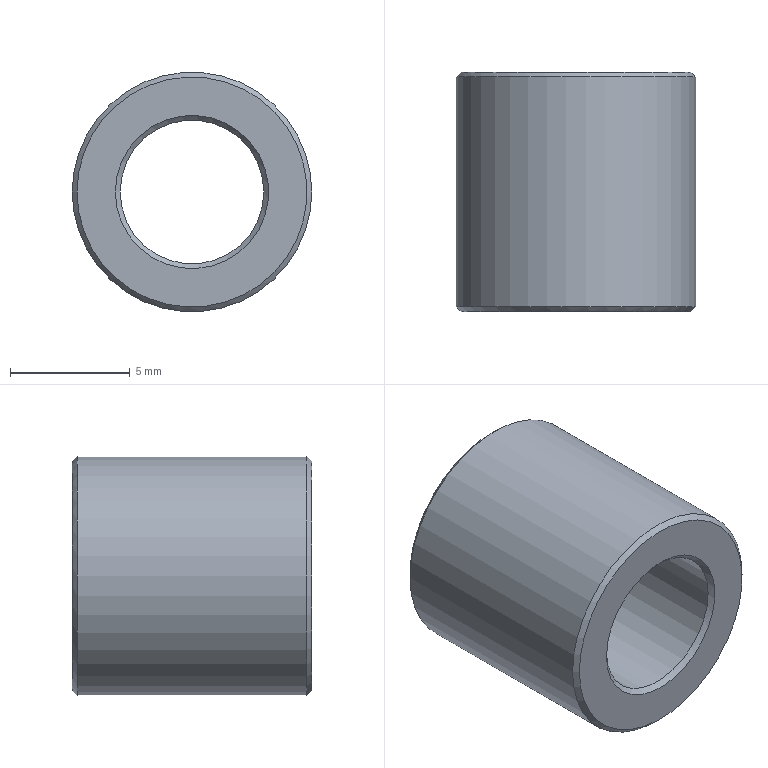Part | NX | features 5003_026_C-KNCLA6-10-10 2 | 1 solid | 8 faces | box 10 x 10 x 10 mm | volume 500.644 mm3 | cone 4 | plane 2 | cylinder 2 | commonest cylinder face diameters 6 x1 10 x1
STEP:
#1=CARTESIAN_POINT('',(-221.575,-608.6,-110.5));
#2=VERTEX_POINT('',#1);
#3=CARTESIAN_POINT('',(-216.775,-608.6,-110.5));
#4=DIRECTION('',(0.,1.,0.));
#5=DIRECTION('',(-1.,0.,0.));
#6=AXIS2_PLACEMENT_3D('',#3,#4,#5);
#7=CIRCLE('',#6,4.8);
#8=EDGE_CURVE('',#2,#2,#7,.F.);
#9=ORIENTED_EDGE('',*,*,#8,.T.);
#10=EDGE_LOOP('',(#9));
#11=FACE_BOUND('',#10,.T.);
#12=CARTESIAN_POINT('',(-219.975,-608.6,-110.5));
#13=VERTEX_POINT('',#12);
#14=CARTESIAN_POINT('',(-216.775,-608.6,-110.5));
#15=DIRECTION('',(0.,1.,0.));
#16=DIRECTION('',(-1.,0.,0.));
#17=AXIS2_PLACEMENT_3D('',#14,#15,#16);
#18=CIRCLE('',#17,3.2);
#19=EDGE_CURVE('',#13,#13,#18,.T.);
#20=ORIENTED_EDGE('',*,*,#19,.T.);
#21=EDGE_LOOP('',(#20));
#22=FACE_BOUND('',#21,.T.);
#23=CARTESIAN_POINT('',(-219.775,-608.6,-110.5));
#24=DIRECTION('',(0.,1.,0.));
#25=DIRECTION('',(-1.,0.,0.));
#26=AXIS2_PLACEMENT_3D('',#23,#24,#25);
#27=PLANE('',#26);
#28=ADVANCED_FACE('',(#11,#22),#27,.F.);
#29=CARTESIAN_POINT('',(-221.775,-608.4,-110.5));
#30=VERTEX_POINT('',#29);
#31=CARTESIAN_POINT('',(-216.775,-608.4,-110.5));
#32=DIRECTION('',(0.,1.,0.));
#33=DIRECTION('',(-1.,0.,0.));
#34=AXIS2_PLACEMENT_3D('',#31,#32,#33);
#35=CIRCLE('',#34,5.);
#36=EDGE_CURVE('',#30,#30,#35,.T.);
#37=ORIENTED_EDGE('',*,*,#36,.T.);
#38=EDGE_LOOP('',(#37));
#39=FACE_BOUND('',#38,.T.);
#40=CARTESIAN_POINT('',(-211.775,-598.8,-110.5));
#41=VERTEX_POINT('',#40);
#42=CARTESIAN_POINT('',(-216.775,-598.8,-110.5));
#43=DIRECTION('',(0.,-1.,0.));
#44=DIRECTION('',(1.,0.,0.));
#45=AXIS2_PLACEMENT_3D('',#42,#43,#44);
#46=CIRCLE('',#45,5.);
#47=EDGE_CURVE('',#41,#41,#46,.T.);
#48=ORIENTED_EDGE('',*,*,#47,.T.);
#49=EDGE_LOOP('',(#48));
#50=FACE_BOUND('',#49,.T.);
#51=CARTESIAN_POINT('',(-216.775,-608.6,-110.5));
#52=DIRECTION('',(0.,-1.,0.));
#53=DIRECTION('',(1.,0.,0.));
#54=AXIS2_PLACEMENT_3D('',#51,#52,#53);
#55=CYLINDRICAL_SURFACE('',#54,5.);
#56=ADVANCED_FACE('',(#39,#50),#55,.T.);
#57=CARTESIAN_POINT('',(-213.575,-598.6,-110.5));
#58=VERTEX_POINT('',#57);
#59=CARTESIAN_POINT('',(-216.775,-598.6,-110.5));
#60=DIRECTION('',(0.,-1.,0.));
#61=DIRECTION('',(1.,0.,0.));
#62=AXIS2_PLACEMENT_3D('',#59,#60,#61);
#63=CIRCLE('',#62,3.2);
#64=EDGE_CURVE('',#58,#58,#63,.T.);
#65=ORIENTED_EDGE('',*,*,#64,.T.);
#66=EDGE_LOOP('',(#65));
#67=FACE_BOUND('',#66,.T.);
#68=CARTESIAN_POINT('',(-211.975,-598.6,-110.5));
#69=VERTEX_POINT('',#68);
#70=CARTESIAN_POINT('',(-216.775,-598.6,-110.5));
#71=DIRECTION('',(0.,-1.,0.));
#72=DIRECTION('',(1.,0.,0.));
#73=AXIS2_PLACEMENT_3D('',#70,#71,#72);
#74=CIRCLE('',#73,4.8);
#75=EDGE_CURVE('',#69,#69,#74,.F.);
#76=ORIENTED_EDGE('',*,*,#75,.T.);
#77=EDGE_LOOP('',(#76));
#78=FACE_BOUND('',#77,.T.);
#79=CARTESIAN_POINT('',(-219.775,-598.6,-110.5));
#80=DIRECTION('',(0.,-1.,0.));
#81=DIRECTION('',(1.,0.,0.));
#82=AXIS2_PLACEMENT_3D('',#79,#80,#81);
#83=PLANE('',#82);
#84=ADVANCED_FACE('',(#67,#78),#83,.F.);
#85=CARTESIAN_POINT('',(-219.775,-608.4,-110.5));
#86=VERTEX_POINT('',#85);
#87=CARTESIAN_POINT('',(-216.775,-608.4,-110.5));
#88=DIRECTION('',(0.,1.,0.));
#89=DIRECTION('',(-1.,0.,0.));
#90=AXIS2_PLACEMENT_3D('',#87,#88,#89);
#91=CIRCLE('',#90,3.);
#92=EDGE_CURVE('',#86,#86,#91,.F.);
#93=ORIENTED_EDGE('',*,*,#92,.T.);
#94=EDGE_LOOP('',(#93));
#95=FACE_BOUND('',#94,.T.);
#96=CARTESIAN_POINT('',(-213.775,-598.8,-110.5));
#97=VERTEX_POINT('',#96);
#98=CARTESIAN_POINT('',(-216.775,-598.8,-110.5));
#99=DIRECTION('',(0.,-1.,0.));
#100=DIRECTION('',(1.,0.,0.));
#101=AXIS2_PLACEMENT_3D('',#98,#99,#100);
#102=CIRCLE('',#101,3.);
#103=EDGE_CURVE('',#97,#97,#102,.F.);
#104=ORIENTED_EDGE('',*,*,#103,.T.);
#105=EDGE_LOOP('',(#104));
#106=FACE_BOUND('',#105,.T.);
#107=CARTESIAN_POINT('',(-216.775,-608.6,-110.5));
#108=DIRECTION('',(0.,-1.,0.));
#109=DIRECTION('',(1.,0.,0.));
#110=AXIS2_PLACEMENT_3D('',#107,#108,#109);
#111=CYLINDRICAL_SURFACE('',#110,3.);
#112=ADVANCED_FACE('',(#95,#106),#111,.F.);
#113=ORIENTED_EDGE('',*,*,#36,.F.);
#114=EDGE_LOOP('',(#113));
#115=FACE_BOUND('',#114,.T.);
#116=ORIENTED_EDGE('',*,*,#8,.F.);
#117=EDGE_LOOP('',(#116));
#118=FACE_BOUND('',#117,.T.);
#119=CARTESIAN_POINT('',(-216.775,-608.6,-110.5));
#120=DIRECTION('',(0.,1.,0.));
#121=DIRECTION('',(-1.,0.,0.));
#122=AXIS2_PLACEMENT_3D('',#119,#120,#121);
#123=CONICAL_SURFACE('',#122,4.8,0.7854);
#124=ADVANCED_FACE('',(#115,#118),#123,.T.);
#125=ORIENTED_EDGE('',*,*,#19,.F.);
#126=EDGE_LOOP('',(#125));
#127=FACE_BOUND('',#126,.T.);
#128=ORIENTED_EDGE('',*,*,#92,.F.);
#129=EDGE_LOOP('',(#128));
#130=FACE_BOUND('',#129,.T.);
#131=CARTESIAN_POINT('',(-216.775,-608.4,-110.5));
#132=DIRECTION('',(0.,-1.,0.));
#133=DIRECTION('',(1.,0.,0.));
#134=AXIS2_PLACEMENT_3D('',#131,#132,#133);
#135=CONICAL_SURFACE('',#134,3.,0.7854);
#136=ADVANCED_FACE('',(#127,#130),#135,.F.);
#137=ORIENTED_EDGE('',*,*,#103,.F.);
#138=EDGE_LOOP('',(#137));
#139=FACE_BOUND('',#138,.T.);
#140=ORIENTED_EDGE('',*,*,#64,.F.);
#141=EDGE_LOOP('',(#140));
#142=FACE_BOUND('',#141,.T.);
#143=CARTESIAN_POINT('',(-216.775,-598.6,-110.5));
#144=DIRECTION('',(0.,1.,0.));
#145=DIRECTION('',(-1.,0.,0.));
#146=AXIS2_PLACEMENT_3D('',#143,#144,#145);
#147=CONICAL_SURFACE('',#146,3.2,0.7854);
#148=ADVANCED_FACE('',(#139,#142),#147,.F.);
#149=ORIENTED_EDGE('',*,*,#75,.F.);
#150=EDGE_LOOP('',(#149));
#151=FACE_BOUND('',#150,.T.);
#152=ORIENTED_EDGE('',*,*,#47,.F.);
#153=EDGE_LOOP('',(#152));
#154=FACE_BOUND('',#153,.T.);
#155=CARTESIAN_POINT('',(-216.775,-598.8,-110.5));
#156=DIRECTION('',(0.,-1.,0.));
#157=DIRECTION('',(1.,0.,0.));
#158=AXIS2_PLACEMENT_3D('',#155,#156,#157);
#159=CONICAL_SURFACE('',#158,5.,0.7854);
#160=ADVANCED_FACE('',(#151,#154),#159,.T.);
#161=CLOSED_SHELL('',(#28,#56,#84,#112,#124,#136,#148,#160));
#162=MANIFOLD_SOLID_BREP('',#161);
#163=(LENGTH_UNIT()NAMED_UNIT(*)SI_UNIT(.MILLI.,.METRE.));
#164=UNCERTAINTY_MEASURE_WITH_UNIT(LENGTH_MEASURE(0.00001),#163,'','');
#165=(NAMED_UNIT(*)PLANE_ANGLE_UNIT()SI_UNIT($,.RADIAN.));
#166=(NAMED_UNIT(*)SI_UNIT($,.STERADIAN.)SOLID_ANGLE_UNIT());
#167=(GEOMETRIC_REPRESENTATION_CONTEXT(3)GLOBAL_UNCERTAINTY_ASSIGNED_CONTEXT((#164))GLOBAL_UNIT_ASSIGNED_CONTEXT((#163,#165,#166))REPRESENTATION_CONTEXT('',''));
#168=ADVANCED_BREP_SHAPE_REPRESENTATION('',(#162),#167);